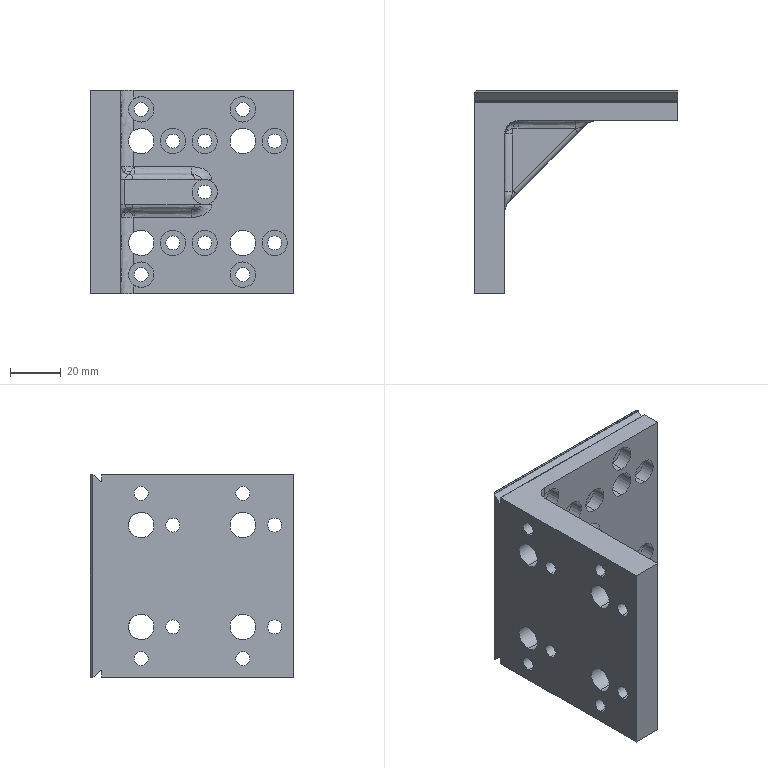Part | STEP file | 00363089_WINKEL_HMB-..._1 | 1 solid | 178 faces | box 80 x 80 x 80 mm | volume 130537 mm3 | cylinder 106 | plane 41 | spline 31 | commonest cylinder face diameters 10 x54 5.5 x38 0.4 x10 9 x4